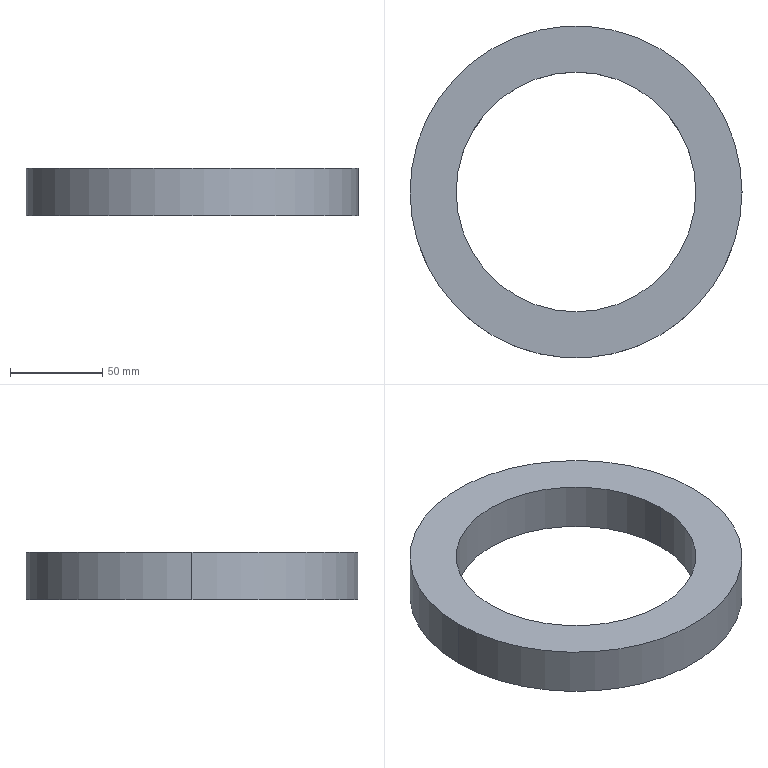Part | SolidWorks | features Extrusion 1 | 1 solid | 6 faces | box 180 x 180 x 26 mm | volume 316515 mm3 | cylinder 4 | plane 2 | commonest cylinder face diameters 130 x2 180 x2
STEP:
#1=CARTESIAN_POINT('',(-65.,0.,26.));
#2=VERTEX_POINT('',#1);
#3=CARTESIAN_POINT('',(65.,0.,26.));
#4=VERTEX_POINT('',#3);
#5=CARTESIAN_POINT('',(0.,0.,26.));
#6=DIRECTION('',(0.,0.,1.));
#7=DIRECTION('',(1.,0.,0.));
#8=AXIS2_PLACEMENT_3D('',#5,#6,#7);
#9=CIRCLE('',#8,65.);
#10=EDGE_CURVE('',#2,#4,#9,.T.);
#11=ORIENTED_EDGE('',*,*,#10,.T.);
#12=CARTESIAN_POINT('',(65.,0.,0.));
#13=VERTEX_POINT('',#12);
#14=CARTESIAN_POINT('',(65.,0.,26.));
#15=DIRECTION('',(0.,0.,-1.));
#16=VECTOR('',#15,1000.);
#17=LINE('',#14,#16);
#18=EDGE_CURVE('',#4,#13,#17,.T.);
#19=ORIENTED_EDGE('',*,*,#18,.T.);
#20=CARTESIAN_POINT('',(-65.,0.,0.));
#21=VERTEX_POINT('',#20);
#22=CARTESIAN_POINT('',(0.,0.,0.));
#23=DIRECTION('',(0.,0.,1.));
#24=DIRECTION('',(1.,0.,0.));
#25=AXIS2_PLACEMENT_3D('',#22,#23,#24);
#26=CIRCLE('',#25,65.);
#27=EDGE_CURVE('',#21,#13,#26,.T.);
#28=ORIENTED_EDGE('',*,*,#27,.F.);
#29=CARTESIAN_POINT('',(-65.,0.,26.));
#30=DIRECTION('',(0.,0.,-1.));
#31=VECTOR('',#30,1000.);
#32=LINE('',#29,#31);
#33=EDGE_CURVE('',#2,#21,#32,.T.);
#34=ORIENTED_EDGE('',*,*,#33,.F.);
#35=EDGE_LOOP('',(#11,#19,#28,#34));
#36=FACE_OUTER_BOUND('',#35,.T.);
#37=CARTESIAN_POINT('',(0.,0.,26.));
#38=DIRECTION('',(0.,0.,-1.));
#39=DIRECTION('',(-1.,0.,0.));
#40=AXIS2_PLACEMENT_3D('',#37,#38,#39);
#41=CYLINDRICAL_SURFACE('',#40,65.);
#42=ADVANCED_FACE('',(#36),#41,.F.);
#43=CARTESIAN_POINT('',(90.,0.,26.));
#44=VERTEX_POINT('',#43);
#45=CARTESIAN_POINT('',(-90.,0.,26.));
#46=VERTEX_POINT('',#45);
#47=CARTESIAN_POINT('',(0.,0.,26.));
#48=DIRECTION('',(0.,0.,1.));
#49=DIRECTION('',(1.,0.,0.));
#50=AXIS2_PLACEMENT_3D('',#47,#48,#49);
#51=CIRCLE('',#50,90.);
#52=EDGE_CURVE('',#44,#46,#51,.T.);
#53=ORIENTED_EDGE('',*,*,#52,.F.);
#54=CARTESIAN_POINT('',(90.,0.,0.));
#55=VERTEX_POINT('',#54);
#56=CARTESIAN_POINT('',(90.,0.,26.));
#57=DIRECTION('',(0.,0.,-1.));
#58=VECTOR('',#57,1000.);
#59=LINE('',#56,#58);
#60=EDGE_CURVE('',#44,#55,#59,.T.);
#61=ORIENTED_EDGE('',*,*,#60,.T.);
#62=CARTESIAN_POINT('',(-90.,0.,0.));
#63=VERTEX_POINT('',#62);
#64=CARTESIAN_POINT('',(0.,0.,0.));
#65=DIRECTION('',(0.,0.,1.));
#66=DIRECTION('',(1.,0.,0.));
#67=AXIS2_PLACEMENT_3D('',#64,#65,#66);
#68=CIRCLE('',#67,90.);
#69=EDGE_CURVE('',#55,#63,#68,.T.);
#70=ORIENTED_EDGE('',*,*,#69,.T.);
#71=CARTESIAN_POINT('',(-90.,0.,26.));
#72=DIRECTION('',(0.,0.,-1.));
#73=VECTOR('',#72,1000.);
#74=LINE('',#71,#73);
#75=EDGE_CURVE('',#46,#63,#74,.T.);
#76=ORIENTED_EDGE('',*,*,#75,.F.);
#77=EDGE_LOOP('',(#53,#61,#70,#76));
#78=FACE_OUTER_BOUND('',#77,.T.);
#79=CARTESIAN_POINT('',(0.,0.,26.));
#80=DIRECTION('',(0.,0.,-1.));
#81=DIRECTION('',(-1.,0.,0.));
#82=AXIS2_PLACEMENT_3D('',#79,#80,#81);
#83=CYLINDRICAL_SURFACE('',#82,90.);
#84=ADVANCED_FACE('',(#78),#83,.T.);
#85=CARTESIAN_POINT('',(0.,0.,26.));
#86=DIRECTION('',(0.,0.,1.));
#87=DIRECTION('',(1.,0.,0.));
#88=AXIS2_PLACEMENT_3D('',#85,#86,#87);
#89=CIRCLE('',#88,90.);
#90=EDGE_CURVE('',#46,#44,#89,.T.);
#91=ORIENTED_EDGE('',*,*,#90,.T.);
#92=ORIENTED_EDGE('',*,*,#52,.T.);
#93=EDGE_LOOP('',(#91,#92));
#94=FACE_OUTER_BOUND('',#93,.T.);
#95=ORIENTED_EDGE('',*,*,#10,.F.);
#96=CARTESIAN_POINT('',(0.,0.,26.));
#97=DIRECTION('',(0.,0.,1.));
#98=DIRECTION('',(1.,0.,0.));
#99=AXIS2_PLACEMENT_3D('',#96,#97,#98);
#100=CIRCLE('',#99,65.);
#101=EDGE_CURVE('',#4,#2,#100,.T.);
#102=ORIENTED_EDGE('',*,*,#101,.F.);
#103=EDGE_LOOP('',(#95,#102));
#104=FACE_BOUND('',#103,.T.);
#105=CARTESIAN_POINT('',(0.,0.,26.));
#106=DIRECTION('',(0.,0.,1.));
#107=DIRECTION('',(1.,0.,0.));
#108=AXIS2_PLACEMENT_3D('',#105,#106,#107);
#109=PLANE('',#108);
#110=ADVANCED_FACE('',(#94,#104),#109,.T.);
#111=CARTESIAN_POINT('',(0.,0.,0.));
#112=DIRECTION('',(0.,0.,1.));
#113=DIRECTION('',(1.,0.,0.));
#114=AXIS2_PLACEMENT_3D('',#111,#112,#113);
#115=CIRCLE('',#114,90.);
#116=EDGE_CURVE('',#63,#55,#115,.T.);
#117=ORIENTED_EDGE('',*,*,#116,.F.);
#118=ORIENTED_EDGE('',*,*,#69,.F.);
#119=EDGE_LOOP('',(#117,#118));
#120=FACE_OUTER_BOUND('',#119,.T.);
#121=ORIENTED_EDGE('',*,*,#27,.T.);
#122=CARTESIAN_POINT('',(0.,0.,0.));
#123=DIRECTION('',(0.,0.,1.));
#124=DIRECTION('',(1.,0.,0.));
#125=AXIS2_PLACEMENT_3D('',#122,#123,#124);
#126=CIRCLE('',#125,65.);
#127=EDGE_CURVE('',#13,#21,#126,.T.);
#128=ORIENTED_EDGE('',*,*,#127,.T.);
#129=EDGE_LOOP('',(#121,#128));
#130=FACE_BOUND('',#129,.T.);
#131=CARTESIAN_POINT('',(0.,0.,0.));
#132=DIRECTION('',(0.,0.,1.));
#133=DIRECTION('',(1.,0.,0.));
#134=AXIS2_PLACEMENT_3D('',#131,#132,#133);
#135=PLANE('',#134);
#136=ADVANCED_FACE('',(#120,#130),#135,.F.);
#137=ORIENTED_EDGE('',*,*,#60,.F.);
#138=ORIENTED_EDGE('',*,*,#90,.F.);
#139=ORIENTED_EDGE('',*,*,#75,.T.);
#140=ORIENTED_EDGE('',*,*,#116,.T.);
#141=EDGE_LOOP('',(#137,#138,#139,#140));
#142=FACE_OUTER_BOUND('',#141,.T.);
#143=CARTESIAN_POINT('',(0.,0.,26.));
#144=DIRECTION('',(0.,0.,-1.));
#145=DIRECTION('',(-1.,0.,0.));
#146=AXIS2_PLACEMENT_3D('',#143,#144,#145);
#147=CYLINDRICAL_SURFACE('',#146,90.);
#148=ADVANCED_FACE('',(#142),#147,.T.);
#149=ORIENTED_EDGE('',*,*,#18,.F.);
#150=ORIENTED_EDGE('',*,*,#101,.T.);
#151=ORIENTED_EDGE('',*,*,#33,.T.);
#152=ORIENTED_EDGE('',*,*,#127,.F.);
#153=EDGE_LOOP('',(#149,#150,#151,#152));
#154=FACE_OUTER_BOUND('',#153,.T.);
#155=CARTESIAN_POINT('',(0.,0.,26.));
#156=DIRECTION('',(0.,0.,-1.));
#157=DIRECTION('',(-1.,0.,0.));
#158=AXIS2_PLACEMENT_3D('',#155,#156,#157);
#159=CYLINDRICAL_SURFACE('',#158,65.);
#160=ADVANCED_FACE('',(#154),#159,.F.);
#161=CLOSED_SHELL('',(#42,#84,#110,#136,#148,#160));
#162=MANIFOLD_SOLID_BREP('',#161);
#163=CARTESIAN_POINT('',(0.,0.,0.));
#164=DIRECTION('',(0.,0.,1.));
#165=DIRECTION('',(1.,0.,0.));
#166=AXIS2_PLACEMENT_3D('',#163,#164,#165);
#167=(LENGTH_UNIT()NAMED_UNIT(*)SI_UNIT(.MILLI.,.METRE.));
#168=UNCERTAINTY_MEASURE_WITH_UNIT(LENGTH_MEASURE(0.00001),#167,'','');
#169=(NAMED_UNIT(*)PLANE_ANGLE_UNIT()SI_UNIT($,.RADIAN.));
#170=(NAMED_UNIT(*)SI_UNIT($,.STERADIAN.)SOLID_ANGLE_UNIT());
#171=(GEOMETRIC_REPRESENTATION_CONTEXT(3)GLOBAL_UNCERTAINTY_ASSIGNED_CONTEXT((#168))GLOBAL_UNIT_ASSIGNED_CONTEXT((#167,#169,#170))REPRESENTATION_CONTEXT('',''));
#172=ADVANCED_BREP_SHAPE_REPRESENTATION('',(#162,#166),#171);